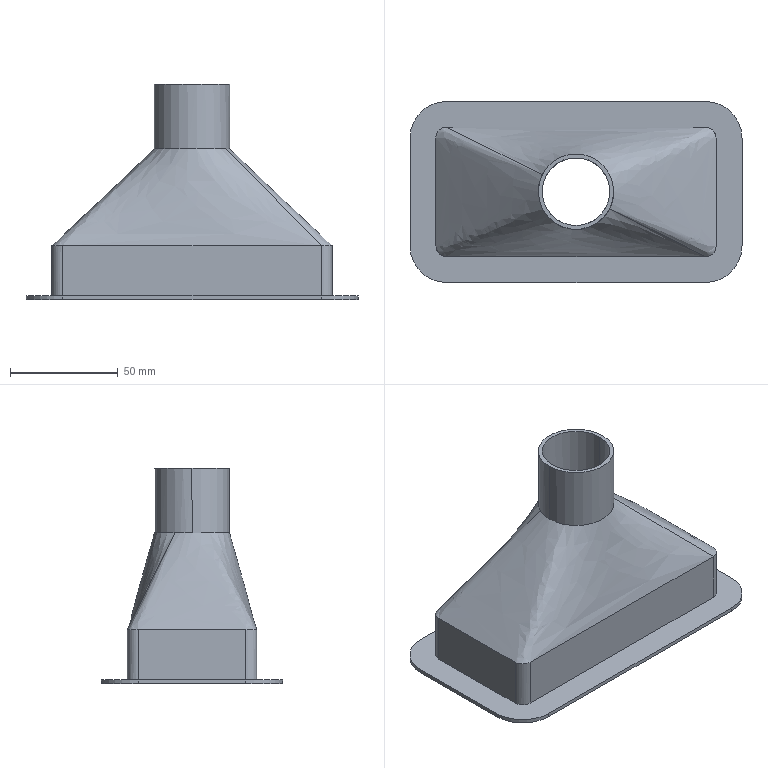Part | SolidWorks | features ICE 2, Blend 1, Extrusion 1, Shell 1 | 1 solid | 35 faces | box 154 x 84 x 100 mm | volume 51797 mm3 | cylinder 16 | plane 15 | spline 4 | commonest cylinder face diameters 6.4 x4 10 x4 34 x4 31.4 x2 35 x2